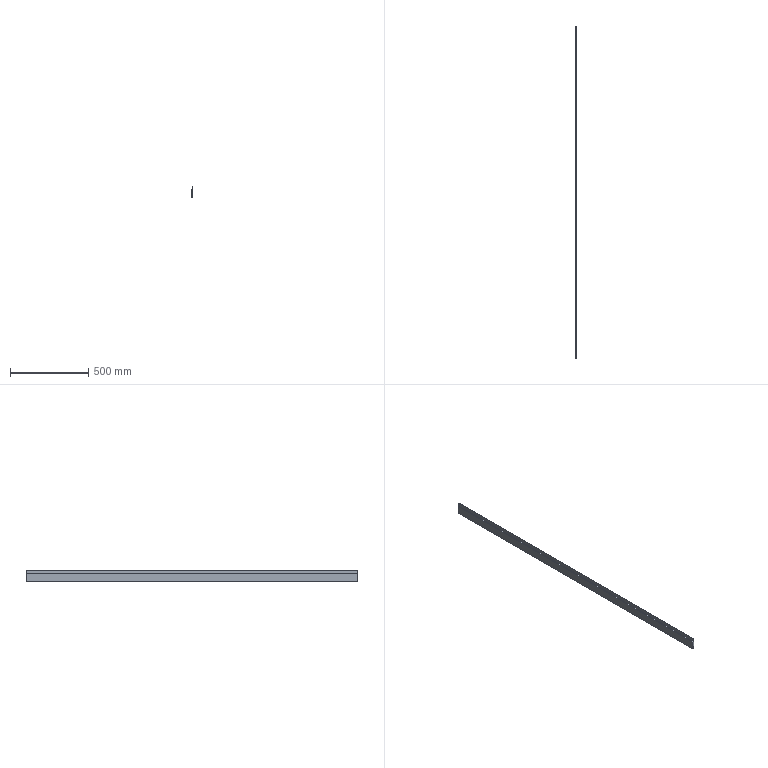Part | NX | features solid 2 | 1 solid | 14 faces | box 10.5 x 2125 x 73.24 mm | volume 1257536 mm3 | plane 8 | cylinder 6 | commonest cylinder face diameters 0.5 x5 1 x1
STEP:
#1=CARTESIAN_POINT('',(-3.,9.35,-1010.56));
#2=VERTEX_POINT('',#1);
#3=CARTESIAN_POINT('',(-3.,9.35,-1030.66));
#4=VERTEX_POINT('',#3);
#5=CARTESIAN_POINT('',(-3.,9.35,-1010.56));
#6=DIRECTION('',(0.,0.,-1.));
#7=VECTOR('',#6,1000.);
#8=LINE('',#5,#7);
#9=EDGE_CURVE('',#2,#4,#8,.T.);
#10=ORIENTED_EDGE('',*,*,#9,.T.);
#11=CARTESIAN_POINT('',(-3.5,9.35,-1031.16));
#12=VERTEX_POINT('',#11);
#13=CARTESIAN_POINT('',(-3.5,9.35,-1030.66));
#14=DIRECTION('',(0.,-1.,0.));
#15=DIRECTION('',(0.,0.,-1.));
#16=AXIS2_PLACEMENT_3D('',#13,#14,#15);
#17=CIRCLE('',#16,0.5);
#18=EDGE_CURVE('',#12,#4,#17,.T.);
#19=ORIENTED_EDGE('',*,*,#18,.F.);
#20=CARTESIAN_POINT('',(-11.25,9.35,-1031.16));
#21=VERTEX_POINT('',#20);
#22=CARTESIAN_POINT('',(-3.5,9.35,-1031.16));
#23=DIRECTION('',(-1.,0.,0.));
#24=VECTOR('',#23,1000.);
#25=LINE('',#22,#24);
#26=EDGE_CURVE('',#12,#21,#25,.T.);
#27=ORIENTED_EDGE('',*,*,#26,.T.);
#28=CARTESIAN_POINT('',(-11.5,9.35,-1031.41));
#29=VERTEX_POINT('',#28);
#30=CARTESIAN_POINT('',(-11.25,9.35,-1031.41));
#31=DIRECTION('',(0.,1.,0.));
#32=DIRECTION('',(-1.,0.,0.));
#33=AXIS2_PLACEMENT_3D('',#30,#31,#32);
#34=CIRCLE('',#33,0.25);
#35=EDGE_CURVE('',#29,#21,#34,.T.);
#36=ORIENTED_EDGE('',*,*,#35,.F.);
#37=CARTESIAN_POINT('',(-11.5,9.35,-1083.3));
#38=VERTEX_POINT('',#37);
#39=CARTESIAN_POINT('',(-11.5,9.35,-1031.41));
#40=DIRECTION('',(0.,0.,-1.));
#41=VECTOR('',#40,1000.);
#42=LINE('',#39,#41);
#43=EDGE_CURVE('',#29,#38,#42,.T.);
#44=ORIENTED_EDGE('',*,*,#43,.T.);
#45=CARTESIAN_POINT('',(-11.25,9.35,-1083.55));
#46=VERTEX_POINT('',#45);
#47=CARTESIAN_POINT('',(-11.25,9.35,-1083.3));
#48=DIRECTION('',(0.,1.,0.));
#49=DIRECTION('',(0.,0.,-1.));
#50=AXIS2_PLACEMENT_3D('',#47,#48,#49);
#51=CIRCLE('',#50,0.25);
#52=EDGE_CURVE('',#46,#38,#51,.T.);
#53=ORIENTED_EDGE('',*,*,#52,.F.);
#54=CARTESIAN_POINT('',(-1.25,9.35,-1083.55));
#55=VERTEX_POINT('',#54);
#56=CARTESIAN_POINT('',(-11.25,9.35,-1083.55));
#57=DIRECTION('',(1.,0.,0.));
#58=VECTOR('',#57,1000.);
#59=LINE('',#56,#58);
#60=EDGE_CURVE('',#46,#55,#59,.T.);
#61=ORIENTED_EDGE('',*,*,#60,.T.);
#62=CARTESIAN_POINT('',(-1.,9.35,-1083.3));
#63=VERTEX_POINT('',#62);
#64=CARTESIAN_POINT('',(-1.25,9.35,-1083.3));
#65=DIRECTION('',(0.,1.,0.));
#66=DIRECTION('',(1.,0.,0.));
#67=AXIS2_PLACEMENT_3D('',#64,#65,#66);
#68=CIRCLE('',#67,0.25);
#69=EDGE_CURVE('',#63,#55,#68,.T.);
#70=ORIENTED_EDGE('',*,*,#69,.F.);
#71=CARTESIAN_POINT('',(-1.,9.35,-1010.56));
#72=VERTEX_POINT('',#71);
#73=CARTESIAN_POINT('',(-1.,9.35,-1083.3));
#74=DIRECTION('',(0.,0.,1.));
#75=VECTOR('',#74,1000.);
#76=LINE('',#73,#75);
#77=EDGE_CURVE('',#63,#72,#76,.T.);
#78=ORIENTED_EDGE('',*,*,#77,.T.);
#79=CARTESIAN_POINT('',(-1.25,9.35,-1010.31));
#80=VERTEX_POINT('',#79);
#81=CARTESIAN_POINT('',(-1.25,9.35,-1010.56));
#82=DIRECTION('',(0.,1.,0.));
#83=DIRECTION('',(0.,0.,1.));
#84=AXIS2_PLACEMENT_3D('',#81,#82,#83);
#85=CIRCLE('',#84,0.25);
#86=EDGE_CURVE('',#80,#72,#85,.T.);
#87=ORIENTED_EDGE('',*,*,#86,.F.);
#88=CARTESIAN_POINT('',(-2.75,9.35,-1010.31));
#89=VERTEX_POINT('',#88);
#90=CARTESIAN_POINT('',(-1.25,9.35,-1010.31));
#91=DIRECTION('',(-1.,0.,0.));
#92=VECTOR('',#91,1000.);
#93=LINE('',#90,#92);
#94=EDGE_CURVE('',#80,#89,#93,.T.);
#95=ORIENTED_EDGE('',*,*,#94,.T.);
#96=CARTESIAN_POINT('',(-2.75,9.35,-1010.56));
#97=DIRECTION('',(0.,1.,0.));
#98=DIRECTION('',(-1.,0.,0.));
#99=AXIS2_PLACEMENT_3D('',#96,#97,#98);
#100=CIRCLE('',#99,0.25);
#101=EDGE_CURVE('',#2,#89,#100,.T.);
#102=ORIENTED_EDGE('',*,*,#101,.F.);
#103=EDGE_LOOP('',(#10,#19,#27,#36,#44,#53,#61,#70,#78,#87,#95,#102));
#104=FACE_BOUND('',#103,.T.);
#105=CARTESIAN_POINT('',(-1.,9.35,-1031.16));
#106=DIRECTION('',(0.,1.,0.));
#107=DIRECTION('',(1.,0.,0.));
#108=AXIS2_PLACEMENT_3D('',#105,#106,#107);
#109=PLANE('',#108);
#110=ADVANCED_FACE('',(#104),#109,.F.);
#111=CARTESIAN_POINT('',(-2.75,2134.35,-1010.31));
#112=VERTEX_POINT('',#111);
#113=CARTESIAN_POINT('',(-2.75,2134.35,-1010.31));
#114=DIRECTION('',(0.,-1.,0.));
#115=VECTOR('',#114,1000.);
#116=LINE('',#113,#115);
#117=EDGE_CURVE('',#112,#89,#116,.T.);
#118=ORIENTED_EDGE('',*,*,#117,.F.);
#119=CARTESIAN_POINT('',(-3.,2134.35,-1010.56));
#120=VERTEX_POINT('',#119);
#121=CARTESIAN_POINT('',(-2.75,2134.35,-1010.56));
#122=DIRECTION('',(0.,-1.,0.));
#123=DIRECTION('',(0.,0.,1.));
#124=AXIS2_PLACEMENT_3D('',#121,#122,#123);
#125=CIRCLE('',#124,0.25);
#126=EDGE_CURVE('',#112,#120,#125,.T.);
#127=ORIENTED_EDGE('',*,*,#126,.T.);
#128=CARTESIAN_POINT('',(-3.,9.35,-1010.56));
#129=DIRECTION('',(0.,1.,0.));
#130=VECTOR('',#129,1000.);
#131=LINE('',#128,#130);
#132=EDGE_CURVE('',#2,#120,#131,.T.);
#133=ORIENTED_EDGE('',*,*,#132,.F.);
#134=ORIENTED_EDGE('',*,*,#101,.T.);
#135=EDGE_LOOP('',(#118,#127,#133,#134));
#136=FACE_BOUND('',#135,.T.);
#137=CARTESIAN_POINT('',(-2.75,4918.322,-1010.56));
#138=DIRECTION('',(0.,-1.,0.));
#139=DIRECTION('',(0.,0.,-1.));
#140=AXIS2_PLACEMENT_3D('',#137,#138,#139);
#141=CYLINDRICAL_SURFACE('',#140,0.25);
#142=ADVANCED_FACE('',(#136),#141,.T.);
#143=CARTESIAN_POINT('',(-3.,2134.35,-1030.66));
#144=VERTEX_POINT('',#143);
#145=CARTESIAN_POINT('',(-3.,2134.35,-1010.56));
#146=DIRECTION('',(0.,0.,-1.));
#147=VECTOR('',#146,1000.);
#148=LINE('',#145,#147);
#149=EDGE_CURVE('',#120,#144,#148,.T.);
#150=ORIENTED_EDGE('',*,*,#149,.T.);
#151=CARTESIAN_POINT('',(-3.,2134.35,-1030.66));
#152=DIRECTION('',(0.,-1.,0.));
#153=VECTOR('',#152,1000.);
#154=LINE('',#151,#153);
#155=EDGE_CURVE('',#144,#4,#154,.T.);
#156=ORIENTED_EDGE('',*,*,#155,.T.);
#157=ORIENTED_EDGE('',*,*,#9,.F.);
#158=ORIENTED_EDGE('',*,*,#132,.T.);
#159=EDGE_LOOP('',(#150,#156,#157,#158));
#160=FACE_BOUND('',#159,.T.);
#161=CARTESIAN_POINT('',(-3.,9.35,-1031.16));
#162=DIRECTION('',(-1.,0.,0.));
#163=DIRECTION('',(0.,0.,-1.));
#164=AXIS2_PLACEMENT_3D('',#161,#162,#163);
#165=PLANE('',#164);
#166=ADVANCED_FACE('',(#160),#165,.T.);
#167=CARTESIAN_POINT('',(-3.5,2134.35,-1031.16));
#168=VERTEX_POINT('',#167);
#169=CARTESIAN_POINT('',(-3.5,2134.35,-1030.66));
#170=DIRECTION('',(0.,1.,0.));
#171=DIRECTION('',(1.,0.,0.));
#172=AXIS2_PLACEMENT_3D('',#169,#170,#171);
#173=CIRCLE('',#172,0.5);
#174=EDGE_CURVE('',#144,#168,#173,.T.);
#175=ORIENTED_EDGE('',*,*,#174,.T.);
#176=CARTESIAN_POINT('',(-3.5,9.35,-1031.16));
#177=DIRECTION('',(0.,1.,0.));
#178=VECTOR('',#177,1000.);
#179=LINE('',#176,#178);
#180=EDGE_CURVE('',#12,#168,#179,.T.);
#181=ORIENTED_EDGE('',*,*,#180,.F.);
#182=ORIENTED_EDGE('',*,*,#18,.T.);
#183=ORIENTED_EDGE('',*,*,#155,.F.);
#184=EDGE_LOOP('',(#175,#181,#182,#183));
#185=FACE_BOUND('',#184,.T.);
#186=CARTESIAN_POINT('',(-3.5,-2768.622,-1030.66));
#187=DIRECTION('',(0.,1.,0.));
#188=DIRECTION('',(-1.,0.,0.));
#189=AXIS2_PLACEMENT_3D('',#186,#187,#188);
#190=CYLINDRICAL_SURFACE('',#189,0.5);
#191=ADVANCED_FACE('',(#185),#190,.F.);
#192=ORIENTED_EDGE('',*,*,#26,.F.);
#193=ORIENTED_EDGE('',*,*,#180,.T.);
#194=CARTESIAN_POINT('',(-11.25,2134.35,-1031.16));
#195=VERTEX_POINT('',#194);
#196=CARTESIAN_POINT('',(-3.5,2134.35,-1031.16));
#197=DIRECTION('',(-1.,0.,0.));
#198=VECTOR('',#197,1000.);
#199=LINE('',#196,#198);
#200=EDGE_CURVE('',#168,#195,#199,.T.);
#201=ORIENTED_EDGE('',*,*,#200,.T.);
#202=CARTESIAN_POINT('',(-11.25,2134.35,-1031.16));
#203=DIRECTION('',(0.,-1.,0.));
#204=VECTOR('',#203,1000.);
#205=LINE('',#202,#204);
#206=EDGE_CURVE('',#195,#21,#205,.T.);
#207=ORIENTED_EDGE('',*,*,#206,.T.);
#208=EDGE_LOOP('',(#192,#193,#201,#207));
#209=FACE_BOUND('',#208,.T.);
#210=CARTESIAN_POINT('',(-11.5,9.35,-1031.16));
#211=DIRECTION('',(0.,0.,1.));
#212=DIRECTION('',(-1.,0.,0.));
#213=AXIS2_PLACEMENT_3D('',#210,#211,#212);
#214=PLANE('',#213);
#215=ADVANCED_FACE('',(#209),#214,.T.);
#216=ORIENTED_EDGE('',*,*,#206,.F.);
#217=CARTESIAN_POINT('',(-11.5,2134.35,-1031.41));
#218=VERTEX_POINT('',#217);
#219=CARTESIAN_POINT('',(-11.25,2134.35,-1031.41));
#220=DIRECTION('',(0.,-1.,0.));
#221=DIRECTION('',(0.,0.,1.));
#222=AXIS2_PLACEMENT_3D('',#219,#220,#221);
#223=CIRCLE('',#222,0.25);
#224=EDGE_CURVE('',#195,#218,#223,.T.);
#225=ORIENTED_EDGE('',*,*,#224,.T.);
#226=CARTESIAN_POINT('',(-11.5,9.35,-1031.41));
#227=DIRECTION('',(0.,1.,0.));
#228=VECTOR('',#227,1000.);
#229=LINE('',#226,#228);
#230=EDGE_CURVE('',#29,#218,#229,.T.);
#231=ORIENTED_EDGE('',*,*,#230,.F.);
#232=ORIENTED_EDGE('',*,*,#35,.T.);
#233=EDGE_LOOP('',(#216,#225,#231,#232));
#234=FACE_BOUND('',#233,.T.);
#235=CARTESIAN_POINT('',(-11.25,4918.322,-1031.41));
#236=DIRECTION('',(0.,-1.,0.));
#237=DIRECTION('',(0.,0.,-1.));
#238=AXIS2_PLACEMENT_3D('',#235,#236,#237);
#239=CYLINDRICAL_SURFACE('',#238,0.25);
#240=ADVANCED_FACE('',(#234),#239,.T.);
#241=CARTESIAN_POINT('',(-11.5,2134.35,-1083.3));
#242=VERTEX_POINT('',#241);
#243=CARTESIAN_POINT('',(-11.5,2134.35,-1031.41));
#244=DIRECTION('',(0.,0.,-1.));
#245=VECTOR('',#244,1000.);
#246=LINE('',#243,#245);
#247=EDGE_CURVE('',#218,#242,#246,.T.);
#248=ORIENTED_EDGE('',*,*,#247,.T.);
#249=CARTESIAN_POINT('',(-11.5,2134.35,-1083.3));
#250=DIRECTION('',(0.,-1.,0.));
#251=VECTOR('',#250,1000.);
#252=LINE('',#249,#251);
#253=EDGE_CURVE('',#242,#38,#252,.T.);
#254=ORIENTED_EDGE('',*,*,#253,.T.);
#255=ORIENTED_EDGE('',*,*,#43,.F.);
#256=ORIENTED_EDGE('',*,*,#230,.T.);
#257=EDGE_LOOP('',(#248,#254,#255,#256));
#258=FACE_BOUND('',#257,.T.);
#259=CARTESIAN_POINT('',(-11.5,9.35,-1083.55));
#260=DIRECTION('',(-1.,0.,0.));
#261=DIRECTION('',(0.,0.,-1.));
#262=AXIS2_PLACEMENT_3D('',#259,#260,#261);
#263=PLANE('',#262);
#264=ADVANCED_FACE('',(#258),#263,.T.);
#265=ORIENTED_EDGE('',*,*,#253,.F.);
#266=CARTESIAN_POINT('',(-11.25,2134.35,-1083.55));
#267=VERTEX_POINT('',#266);
#268=CARTESIAN_POINT('',(-11.25,2134.35,-1083.3));
#269=DIRECTION('',(0.,-1.,0.));
#270=DIRECTION('',(-1.,0.,0.));
#271=AXIS2_PLACEMENT_3D('',#268,#269,#270);
#272=CIRCLE('',#271,0.25);
#273=EDGE_CURVE('',#242,#267,#272,.T.);
#274=ORIENTED_EDGE('',*,*,#273,.T.);
#275=CARTESIAN_POINT('',(-11.25,9.35,-1083.55));
#276=DIRECTION('',(0.,1.,0.));
#277=VECTOR('',#276,1000.);
#278=LINE('',#275,#277);
#279=EDGE_CURVE('',#46,#267,#278,.T.);
#280=ORIENTED_EDGE('',*,*,#279,.F.);
#281=ORIENTED_EDGE('',*,*,#52,.T.);
#282=EDGE_LOOP('',(#265,#274,#280,#281));
#283=FACE_BOUND('',#282,.T.);
#284=CARTESIAN_POINT('',(-11.25,4918.322,-1083.3));
#285=DIRECTION('',(0.,-1.,0.));
#286=DIRECTION('',(1.,0.,0.));
#287=AXIS2_PLACEMENT_3D('',#284,#285,#286);
#288=CYLINDRICAL_SURFACE('',#287,0.25);
#289=ADVANCED_FACE('',(#283),#288,.T.);
#290=ORIENTED_EDGE('',*,*,#60,.F.);
#291=ORIENTED_EDGE('',*,*,#279,.T.);
#292=CARTESIAN_POINT('',(-1.25,2134.35,-1083.55));
#293=VERTEX_POINT('',#292);
#294=CARTESIAN_POINT('',(-11.25,2134.35,-1083.55));
#295=DIRECTION('',(1.,0.,0.));
#296=VECTOR('',#295,1000.);
#297=LINE('',#294,#296);
#298=EDGE_CURVE('',#267,#293,#297,.T.);
#299=ORIENTED_EDGE('',*,*,#298,.T.);
#300=CARTESIAN_POINT('',(-1.25,2134.35,-1083.55));
#301=DIRECTION('',(0.,-1.,0.));
#302=VECTOR('',#301,1000.);
#303=LINE('',#300,#302);
#304=EDGE_CURVE('',#293,#55,#303,.T.);
#305=ORIENTED_EDGE('',*,*,#304,.T.);
#306=EDGE_LOOP('',(#290,#291,#299,#305));
#307=FACE_BOUND('',#306,.T.);
#308=CARTESIAN_POINT('',(-1.,9.35,-1083.55));
#309=DIRECTION('',(0.,0.,-1.));
#310=DIRECTION('',(1.,0.,0.));
#311=AXIS2_PLACEMENT_3D('',#308,#309,#310);
#312=PLANE('',#311);
#313=ADVANCED_FACE('',(#307),#312,.T.);
#314=ORIENTED_EDGE('',*,*,#304,.F.);
#315=CARTESIAN_POINT('',(-1.,2134.35,-1083.3));
#316=VERTEX_POINT('',#315);
#317=CARTESIAN_POINT('',(-1.25,2134.35,-1083.3));
#318=DIRECTION('',(0.,-1.,0.));
#319=DIRECTION('',(0.,0.,-1.));
#320=AXIS2_PLACEMENT_3D('',#317,#318,#319);
#321=CIRCLE('',#320,0.25);
#322=EDGE_CURVE('',#293,#316,#321,.T.);
#323=ORIENTED_EDGE('',*,*,#322,.T.);
#324=CARTESIAN_POINT('',(-1.,9.35,-1083.3));
#325=DIRECTION('',(0.,1.,0.));
#326=VECTOR('',#325,1000.);
#327=LINE('',#324,#326);
#328=EDGE_CURVE('',#63,#316,#327,.T.);
#329=ORIENTED_EDGE('',*,*,#328,.F.);
#330=ORIENTED_EDGE('',*,*,#69,.T.);
#331=EDGE_LOOP('',(#314,#323,#329,#330));
#332=FACE_BOUND('',#331,.T.);
#333=CARTESIAN_POINT('',(-1.25,4918.322,-1083.3));
#334=DIRECTION('',(0.,-1.,0.));
#335=DIRECTION('',(0.,0.,1.));
#336=AXIS2_PLACEMENT_3D('',#333,#334,#335);
#337=CYLINDRICAL_SURFACE('',#336,0.25);
#338=ADVANCED_FACE('',(#332),#337,.T.);
#339=ORIENTED_EDGE('',*,*,#77,.F.);
#340=ORIENTED_EDGE('',*,*,#328,.T.);
#341=CARTESIAN_POINT('',(-1.,2134.35,-1010.56));
#342=VERTEX_POINT('',#341);
#343=CARTESIAN_POINT('',(-1.,2134.35,-1083.3));
#344=DIRECTION('',(0.,0.,1.));
#345=VECTOR('',#344,1000.);
#346=LINE('',#343,#345);
#347=EDGE_CURVE('',#316,#342,#346,.T.);
#348=ORIENTED_EDGE('',*,*,#347,.T.);
#349=CARTESIAN_POINT('',(-1.,2134.35,-1010.56));
#350=DIRECTION('',(0.,-1.,0.));
#351=VECTOR('',#350,1000.);
#352=LINE('',#349,#351);
#353=EDGE_CURVE('',#342,#72,#352,.T.);
#354=ORIENTED_EDGE('',*,*,#353,.T.);
#355=EDGE_LOOP('',(#339,#340,#348,#354));
#356=FACE_BOUND('',#355,.T.);
#357=CARTESIAN_POINT('',(-1.,9.35,-1010.31));
#358=DIRECTION('',(1.,0.,0.));
#359=DIRECTION('',(0.,0.,1.));
#360=AXIS2_PLACEMENT_3D('',#357,#358,#359);
#361=PLANE('',#360);
#362=ADVANCED_FACE('',(#356),#361,.T.);
#363=ORIENTED_EDGE('',*,*,#353,.F.);
#364=CARTESIAN_POINT('',(-1.25,2134.35,-1010.31));
#365=VERTEX_POINT('',#364);
#366=CARTESIAN_POINT('',(-1.25,2134.35,-1010.56));
#367=DIRECTION('',(0.,-1.,0.));
#368=DIRECTION('',(1.,0.,0.));
#369=AXIS2_PLACEMENT_3D('',#366,#367,#368);
#370=CIRCLE('',#369,0.25);
#371=EDGE_CURVE('',#342,#365,#370,.T.);
#372=ORIENTED_EDGE('',*,*,#371,.T.);
#373=CARTESIAN_POINT('',(-1.25,9.35,-1010.31));
#374=DIRECTION('',(0.,1.,0.));
#375=VECTOR('',#374,1000.);
#376=LINE('',#373,#375);
#377=EDGE_CURVE('',#80,#365,#376,.T.);
#378=ORIENTED_EDGE('',*,*,#377,.F.);
#379=ORIENTED_EDGE('',*,*,#86,.T.);
#380=EDGE_LOOP('',(#363,#372,#378,#379));
#381=FACE_BOUND('',#380,.T.);
#382=CARTESIAN_POINT('',(-1.25,4918.322,-1010.56));
#383=DIRECTION('',(0.,-1.,0.));
#384=DIRECTION('',(-1.,0.,0.));
#385=AXIS2_PLACEMENT_3D('',#382,#383,#384);
#386=CYLINDRICAL_SURFACE('',#385,0.25);
#387=ADVANCED_FACE('',(#381),#386,.T.);
#388=ORIENTED_EDGE('',*,*,#94,.F.);
#389=ORIENTED_EDGE('',*,*,#377,.T.);
#390=CARTESIAN_POINT('',(-1.25,2134.35,-1010.31));
#391=DIRECTION('',(-1.,0.,0.));
#392=VECTOR('',#391,1000.);
#393=LINE('',#390,#392);
#394=EDGE_CURVE('',#365,#112,#393,.T.);
#395=ORIENTED_EDGE('',*,*,#394,.T.);
#396=ORIENTED_EDGE('',*,*,#117,.T.);
#397=EDGE_LOOP('',(#388,#389,#395,#396));
#398=FACE_BOUND('',#397,.T.);
#399=CARTESIAN_POINT('',(-3.,9.35,-1010.31));
#400=DIRECTION('',(0.,0.,1.));
#401=DIRECTION('',(-1.,0.,0.));
#402=AXIS2_PLACEMENT_3D('',#399,#400,#401);
#403=PLANE('',#402);
#404=ADVANCED_FACE('',(#398),#403,.T.);
#405=ORIENTED_EDGE('',*,*,#394,.F.);
#406=ORIENTED_EDGE('',*,*,#371,.F.);
#407=ORIENTED_EDGE('',*,*,#347,.F.);
#408=ORIENTED_EDGE('',*,*,#322,.F.);
#409=ORIENTED_EDGE('',*,*,#298,.F.);
#410=ORIENTED_EDGE('',*,*,#273,.F.);
#411=ORIENTED_EDGE('',*,*,#247,.F.);
#412=ORIENTED_EDGE('',*,*,#224,.F.);
#413=ORIENTED_EDGE('',*,*,#200,.F.);
#414=ORIENTED_EDGE('',*,*,#174,.F.);
#415=ORIENTED_EDGE('',*,*,#149,.F.);
#416=ORIENTED_EDGE('',*,*,#126,.F.);
#417=EDGE_LOOP('',(#405,#406,#407,#408,#409,#410,#411,#412,#413,#414,#415,#416));
#418=FACE_BOUND('',#417,.T.);
#419=CARTESIAN_POINT('',(-1.,2134.35,-1031.16));
#420=DIRECTION('',(0.,1.,0.));
#421=DIRECTION('',(1.,0.,0.));
#422=AXIS2_PLACEMENT_3D('',#419,#420,#421);
#423=PLANE('',#422);
#424=ADVANCED_FACE('',(#418),#423,.T.);
#425=CLOSED_SHELL('',(#110,#142,#166,#191,#215,#240,#264,#289,#313,#338,#362,#387,#404,#424));
#426=MANIFOLD_SOLID_BREP('',#425);
#427=(LENGTH_UNIT()NAMED_UNIT(*)SI_UNIT(.MILLI.,.METRE.));
#428=UNCERTAINTY_MEASURE_WITH_UNIT(LENGTH_MEASURE(0.00001),#427,'','');
#429=(NAMED_UNIT(*)PLANE_ANGLE_UNIT()SI_UNIT($,.RADIAN.));
#430=(NAMED_UNIT(*)SI_UNIT($,.STERADIAN.)SOLID_ANGLE_UNIT());
#431=(GEOMETRIC_REPRESENTATION_CONTEXT(3)GLOBAL_UNCERTAINTY_ASSIGNED_CONTEXT((#428))GLOBAL_UNIT_ASSIGNED_CONTEXT((#427,#429,#430))REPRESENTATION_CONTEXT('',''));
#432=ADVANCED_BREP_SHAPE_REPRESENTATION('',(#426),#431);